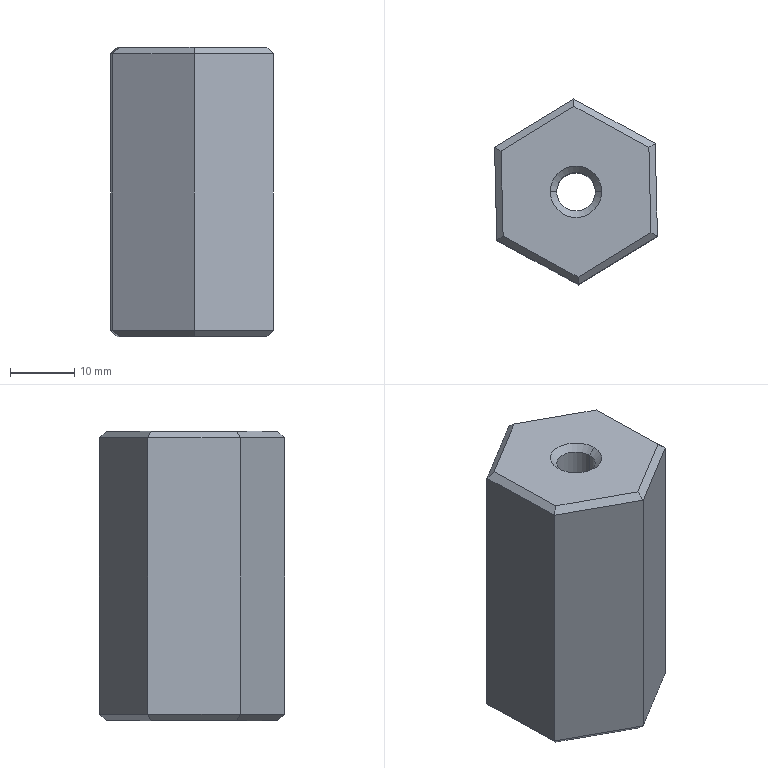Part | STEP file | Sheath | 1 solid | 26 faces | box 25.34 x 28.859 x 45 mm | volume 22979 mm3 | plane 20 | cone 4 | cylinder 2 | commonest cylinder face diameters 6 x2
STEP:
#1=CARTESIAN_POINT('',(3.,0.,1.));
#2=VERTEX_POINT('',#1);
#3=CARTESIAN_POINT('',(-3.,0.,1.));
#4=VERTEX_POINT('',#3);
#5=CARTESIAN_POINT('',(0.,0.,1.));
#6=DIRECTION('',(0.,0.,-1.));
#7=DIRECTION('',(-1.,0.,0.));
#8=AXIS2_PLACEMENT_3D('',#5,#6,#7);
#9=CIRCLE('',#8,3.);
#10=EDGE_CURVE('',#2,#4,#9,.T.);
#11=ORIENTED_EDGE('',*,*,#10,.F.);
#12=CARTESIAN_POINT('',(4.,0.,0.));
#13=VERTEX_POINT('',#12);
#14=CARTESIAN_POINT('',(4.,0.,0.));
#15=DIRECTION('',(0.7071,0.,-0.7071));
#16=VECTOR('',#15,1000.);
#17=LINE('',#14,#16);
#18=EDGE_CURVE('',#2,#13,#17,.T.);
#19=ORIENTED_EDGE('',*,*,#18,.T.);
#20=CARTESIAN_POINT('',(-4.,0.,0.));
#21=VERTEX_POINT('',#20);
#22=CARTESIAN_POINT('',(0.,0.,0.));
#23=DIRECTION('',(0.,0.,-1.));
#24=DIRECTION('',(-1.,0.,0.));
#25=AXIS2_PLACEMENT_3D('',#22,#23,#24);
#26=CIRCLE('',#25,4.);
#27=EDGE_CURVE('',#13,#21,#26,.T.);
#28=ORIENTED_EDGE('',*,*,#27,.T.);
#29=CARTESIAN_POINT('',(-4.,0.,0.));
#30=DIRECTION('',(-0.7071,0.,-0.7071));
#31=VECTOR('',#30,1000.);
#32=LINE('',#29,#31);
#33=EDGE_CURVE('',#4,#21,#32,.T.);
#34=ORIENTED_EDGE('',*,*,#33,.F.);
#35=EDGE_LOOP('',(#11,#19,#28,#34));
#36=FACE_OUTER_BOUND('',#35,.T.);
#37=CARTESIAN_POINT('',(0.,0.,0.));
#38=DIRECTION('',(0.,0.,-1.));
#39=DIRECTION('',(-1.,0.,0.));
#40=AXIS2_PLACEMENT_3D('',#37,#38,#39);
#41=CONICAL_SURFACE('',#40,4.,0.7854);
#42=ADVANCED_FACE('',(#36),#41,.F.);
#43=CARTESIAN_POINT('',(-3.,0.,44.));
#44=VERTEX_POINT('',#43);
#45=CARTESIAN_POINT('',(3.,0.,44.));
#46=VERTEX_POINT('',#45);
#47=CARTESIAN_POINT('',(0.,0.,44.));
#48=DIRECTION('',(0.,0.,1.));
#49=DIRECTION('',(1.,0.,0.));
#50=AXIS2_PLACEMENT_3D('',#47,#48,#49);
#51=CIRCLE('',#50,3.);
#52=EDGE_CURVE('',#44,#46,#51,.T.);
#53=ORIENTED_EDGE('',*,*,#52,.F.);
#54=CARTESIAN_POINT('',(-4.,0.,45.));
#55=VERTEX_POINT('',#54);
#56=CARTESIAN_POINT('',(-4.,0.,45.));
#57=DIRECTION('',(-0.7071,0.,0.7071));
#58=VECTOR('',#57,1000.);
#59=LINE('',#56,#58);
#60=EDGE_CURVE('',#44,#55,#59,.T.);
#61=ORIENTED_EDGE('',*,*,#60,.T.);
#62=CARTESIAN_POINT('',(4.,0.,45.));
#63=VERTEX_POINT('',#62);
#64=CARTESIAN_POINT('',(0.,0.,45.));
#65=DIRECTION('',(0.,0.,-1.));
#66=DIRECTION('',(1.,0.,0.));
#67=AXIS2_PLACEMENT_3D('',#64,#65,#66);
#68=CIRCLE('',#67,4.);
#69=EDGE_CURVE('',#63,#55,#68,.T.);
#70=ORIENTED_EDGE('',*,*,#69,.F.);
#71=CARTESIAN_POINT('',(4.,0.,45.));
#72=DIRECTION('',(0.7071,0.,0.7071));
#73=VECTOR('',#72,1000.);
#74=LINE('',#71,#73);
#75=EDGE_CURVE('',#46,#63,#74,.T.);
#76=ORIENTED_EDGE('',*,*,#75,.F.);
#77=EDGE_LOOP('',(#53,#61,#70,#76));
#78=FACE_OUTER_BOUND('',#77,.T.);
#79=CARTESIAN_POINT('',(0.,0.,45.));
#80=DIRECTION('',(0.,0.,1.));
#81=DIRECTION('',(1.,0.,0.));
#82=AXIS2_PLACEMENT_3D('',#79,#80,#81);
#83=CONICAL_SURFACE('',#82,4.,0.7854);
#84=ADVANCED_FACE('',(#78),#83,.F.);
#85=ORIENTED_EDGE('',*,*,#52,.T.);
#86=CARTESIAN_POINT('',(3.,0.,45.));
#87=DIRECTION('',(0.,0.,-1.));
#88=VECTOR('',#87,1000.);
#89=LINE('',#86,#88);
#90=EDGE_CURVE('',#46,#2,#89,.T.);
#91=ORIENTED_EDGE('',*,*,#90,.T.);
#92=ORIENTED_EDGE('',*,*,#10,.T.);
#93=CARTESIAN_POINT('',(-3.,0.,45.));
#94=DIRECTION('',(0.,0.,-1.));
#95=VECTOR('',#94,1000.);
#96=LINE('',#93,#95);
#97=EDGE_CURVE('',#44,#4,#96,.T.);
#98=ORIENTED_EDGE('',*,*,#97,.F.);
#99=EDGE_LOOP('',(#85,#91,#92,#98));
#100=FACE_OUTER_BOUND('',#99,.T.);
#101=CARTESIAN_POINT('',(0.,0.,45.));
#102=DIRECTION('',(0.,0.,-1.));
#103=DIRECTION('',(-1.,0.,0.));
#104=AXIS2_PLACEMENT_3D('',#101,#102,#103);
#105=CYLINDRICAL_SURFACE('',#104,3.);
#106=ADVANCED_FACE('',(#100),#105,.F.);
#107=CARTESIAN_POINT('',(12.323,7.516,1.));
#108=VERTEX_POINT('',#107);
#109=CARTESIAN_POINT('',(12.67,-6.914,1.));
#110=VERTEX_POINT('',#109);
#111=CARTESIAN_POINT('',(12.67,-6.914,1.));
#112=DIRECTION('',(0.02408,-0.9997,0.));
#113=VECTOR('',#112,1000.);
#114=LINE('',#111,#113);
#115=EDGE_CURVE('',#108,#110,#114,.T.);
#116=ORIENTED_EDGE('',*,*,#115,.F.);
#117=CARTESIAN_POINT('',(12.323,7.516,44.));
#118=VERTEX_POINT('',#117);
#119=CARTESIAN_POINT('',(12.323,7.516,45.));
#120=DIRECTION('',(0.,0.,-1.));
#121=VECTOR('',#120,1000.);
#122=LINE('',#119,#121);
#123=EDGE_CURVE('',#118,#108,#122,.T.);
#124=ORIENTED_EDGE('',*,*,#123,.F.);
#125=CARTESIAN_POINT('',(12.67,-6.914,44.));
#126=VERTEX_POINT('',#125);
#127=CARTESIAN_POINT('',(12.67,-6.914,44.));
#128=DIRECTION('',(-0.02408,0.9997,0.));
#129=VECTOR('',#128,1000.);
#130=LINE('',#127,#129);
#131=EDGE_CURVE('',#126,#118,#130,.T.);
#132=ORIENTED_EDGE('',*,*,#131,.F.);
#133=CARTESIAN_POINT('',(12.67,-6.914,45.));
#134=DIRECTION('',(0.,0.,1.));
#135=VECTOR('',#134,1000.);
#136=LINE('',#133,#135);
#137=EDGE_CURVE('',#110,#126,#136,.T.);
#138=ORIENTED_EDGE('',*,*,#137,.F.);
#139=EDGE_LOOP('',(#116,#124,#132,#138));
#140=FACE_OUTER_BOUND('',#139,.T.);
#141=CARTESIAN_POINT('',(12.67,-6.914,45.));
#142=DIRECTION('',(-0.9997,-0.02408,0.));
#143=DIRECTION('',(0.02408,-0.9997,0.));
#144=AXIS2_PLACEMENT_3D('',#141,#142,#143);
#145=PLANE('',#144);
#146=ADVANCED_FACE('',(#140),#145,.F.);
#147=CARTESIAN_POINT('',(0.3475,-14.43,1.));
#148=VERTEX_POINT('',#147);
#149=CARTESIAN_POINT('',(0.3475,-14.43,1.));
#150=DIRECTION('',(-0.8537,-0.5207,0.));
#151=VECTOR('',#150,1000.);
#152=LINE('',#149,#151);
#153=EDGE_CURVE('',#110,#148,#152,.T.);
#154=ORIENTED_EDGE('',*,*,#153,.F.);
#155=ORIENTED_EDGE('',*,*,#137,.T.);
#156=CARTESIAN_POINT('',(0.3475,-14.43,44.));
#157=VERTEX_POINT('',#156);
#158=CARTESIAN_POINT('',(0.3475,-14.43,44.));
#159=DIRECTION('',(0.8537,0.5207,0.));
#160=VECTOR('',#159,1000.);
#161=LINE('',#158,#160);
#162=EDGE_CURVE('',#157,#126,#161,.T.);
#163=ORIENTED_EDGE('',*,*,#162,.F.);
#164=CARTESIAN_POINT('',(0.3475,-14.43,45.));
#165=DIRECTION('',(0.,0.,1.));
#166=VECTOR('',#165,1000.);
#167=LINE('',#164,#166);
#168=EDGE_CURVE('',#148,#157,#167,.T.);
#169=ORIENTED_EDGE('',*,*,#168,.F.);
#170=EDGE_LOOP('',(#154,#155,#163,#169));
#171=FACE_OUTER_BOUND('',#170,.T.);
#172=CARTESIAN_POINT('',(0.3475,-14.43,45.));
#173=DIRECTION('',(-0.5207,0.8537,0.));
#174=DIRECTION('',(-0.8537,-0.5207,0.));
#175=AXIS2_PLACEMENT_3D('',#172,#173,#174);
#176=PLANE('',#175);
#177=ADVANCED_FACE('',(#171),#176,.F.);
#178=CARTESIAN_POINT('',(11.337,6.914,0.));
#179=VERTEX_POINT('',#178);
#180=CARTESIAN_POINT('',(11.657,-6.361,0.));
#181=VERTEX_POINT('',#180);
#182=CARTESIAN_POINT('',(11.337,6.914,0.));
#183=DIRECTION('',(0.02408,-0.9997,0.));
#184=VECTOR('',#183,1000.);
#185=LINE('',#182,#184);
#186=EDGE_CURVE('',#179,#181,#185,.T.);
#187=ORIENTED_EDGE('',*,*,#186,.F.);
#188=CARTESIAN_POINT('',(11.337,6.914,0.));
#189=DIRECTION('',(0.6454,0.3936,0.6547));
#190=VECTOR('',#189,1000.);
#191=LINE('',#188,#190);
#192=EDGE_CURVE('',#179,#108,#191,.T.);
#193=ORIENTED_EDGE('',*,*,#192,.T.);
#194=ORIENTED_EDGE('',*,*,#115,.T.);
#195=CARTESIAN_POINT('',(11.657,-6.361,0.));
#196=DIRECTION('',(0.6636,-0.3621,0.6547));
#197=VECTOR('',#196,1000.);
#198=LINE('',#195,#197);
#199=EDGE_CURVE('',#181,#110,#198,.T.);
#200=ORIENTED_EDGE('',*,*,#199,.F.);
#201=EDGE_LOOP('',(#187,#193,#194,#200));
#202=FACE_OUTER_BOUND('',#201,.T.);
#203=CARTESIAN_POINT('',(12.67,-6.914,1.));
#204=DIRECTION('',(-0.7069,-0.01702,0.7071));
#205=DIRECTION('',(0.7072,0.,0.707));
#206=AXIS2_PLACEMENT_3D('',#203,#204,#205);
#207=PLANE('',#206);
#208=ADVANCED_FACE('',(#202),#207,.F.);
#209=CARTESIAN_POINT('',(-0.3475,14.43,1.));
#210=VERTEX_POINT('',#209);
#211=CARTESIAN_POINT('',(12.323,7.516,1.));
#212=DIRECTION('',(0.8778,-0.479,0.));
#213=VECTOR('',#212,1000.);
#214=LINE('',#211,#213);
#215=EDGE_CURVE('',#210,#108,#214,.T.);
#216=ORIENTED_EDGE('',*,*,#215,.F.);
#217=CARTESIAN_POINT('',(-0.3475,14.43,44.));
#218=VERTEX_POINT('',#217);
#219=CARTESIAN_POINT('',(-0.3475,14.43,45.));
#220=DIRECTION('',(0.,0.,-1.));
#221=VECTOR('',#220,1000.);
#222=LINE('',#219,#221);
#223=EDGE_CURVE('',#218,#210,#222,.T.);
#224=ORIENTED_EDGE('',*,*,#223,.F.);
#225=CARTESIAN_POINT('',(12.323,7.516,44.));
#226=DIRECTION('',(-0.8778,0.479,0.));
#227=VECTOR('',#226,1000.);
#228=LINE('',#225,#227);
#229=EDGE_CURVE('',#118,#218,#228,.T.);
#230=ORIENTED_EDGE('',*,*,#229,.F.);
#231=ORIENTED_EDGE('',*,*,#123,.T.);
#232=EDGE_LOOP('',(#216,#224,#230,#231));
#233=FACE_OUTER_BOUND('',#232,.T.);
#234=CARTESIAN_POINT('',(12.323,7.516,45.));
#235=DIRECTION('',(-0.479,-0.8778,0.));
#236=DIRECTION('',(0.8778,-0.479,0.));
#237=AXIS2_PLACEMENT_3D('',#234,#235,#236);
#238=PLANE('',#237);
#239=ADVANCED_FACE('',(#233),#238,.F.);
#240=CARTESIAN_POINT('',(11.657,-6.361,45.));
#241=VERTEX_POINT('',#240);
#242=CARTESIAN_POINT('',(11.657,-6.361,45.));
#243=DIRECTION('',(0.6636,-0.3621,-0.6547));
#244=VECTOR('',#243,1000.);
#245=LINE('',#242,#244);
#246=EDGE_CURVE('',#241,#126,#245,.T.);
#247=ORIENTED_EDGE('',*,*,#246,.T.);
#248=ORIENTED_EDGE('',*,*,#131,.T.);
#249=CARTESIAN_POINT('',(11.337,6.914,45.));
#250=VERTEX_POINT('',#249);
#251=CARTESIAN_POINT('',(12.323,7.516,44.));
#252=DIRECTION('',(-0.6454,-0.3936,0.6547));
#253=VECTOR('',#252,1000.);
#254=LINE('',#251,#253);
#255=EDGE_CURVE('',#118,#250,#254,.T.);
#256=ORIENTED_EDGE('',*,*,#255,.T.);
#257=CARTESIAN_POINT('',(11.337,6.914,45.));
#258=DIRECTION('',(0.02408,-0.9997,0.));
#259=VECTOR('',#258,1000.);
#260=LINE('',#257,#259);
#261=EDGE_CURVE('',#250,#241,#260,.T.);
#262=ORIENTED_EDGE('',*,*,#261,.T.);
#263=EDGE_LOOP('',(#247,#248,#256,#262));
#264=FACE_OUTER_BOUND('',#263,.T.);
#265=CARTESIAN_POINT('',(11.67,-6.938,45.));
#266=DIRECTION('',(0.7069,0.01702,0.7071));
#267=DIRECTION('',(0.7072,0.,-0.707));
#268=AXIS2_PLACEMENT_3D('',#265,#266,#267);
#269=PLANE('',#268);
#270=ADVANCED_FACE('',(#264),#269,.T.);
#271=CARTESIAN_POINT('',(-12.323,-7.516,1.));
#272=VERTEX_POINT('',#271);
#273=CARTESIAN_POINT('',(-12.323,-7.516,1.));
#274=DIRECTION('',(-0.8778,0.479,0.));
#275=VECTOR('',#274,1000.);
#276=LINE('',#273,#275);
#277=EDGE_CURVE('',#148,#272,#276,.T.);
#278=ORIENTED_EDGE('',*,*,#277,.F.);
#279=ORIENTED_EDGE('',*,*,#168,.T.);
#280=CARTESIAN_POINT('',(-12.323,-7.516,44.));
#281=VERTEX_POINT('',#280);
#282=CARTESIAN_POINT('',(-12.323,-7.516,44.));
#283=DIRECTION('',(0.8778,-0.479,0.));
#284=VECTOR('',#283,1000.);
#285=LINE('',#282,#284);
#286=EDGE_CURVE('',#281,#157,#285,.T.);
#287=ORIENTED_EDGE('',*,*,#286,.F.);
#288=CARTESIAN_POINT('',(-12.323,-7.516,45.));
#289=DIRECTION('',(0.,0.,1.));
#290=VECTOR('',#289,1000.);
#291=LINE('',#288,#290);
#292=EDGE_CURVE('',#272,#281,#291,.T.);
#293=ORIENTED_EDGE('',*,*,#292,.F.);
#294=EDGE_LOOP('',(#278,#279,#287,#293));
#295=FACE_OUTER_BOUND('',#294,.T.);
#296=CARTESIAN_POINT('',(-12.323,-7.516,45.));
#297=DIRECTION('',(0.479,0.8778,0.));
#298=DIRECTION('',(-0.8778,0.479,0.));
#299=AXIS2_PLACEMENT_3D('',#296,#297,#298);
#300=PLANE('',#299);
#301=ADVANCED_FACE('',(#295),#300,.F.);
#302=CARTESIAN_POINT('',(0.3197,-13.275,0.));
#303=VERTEX_POINT('',#302);
#304=CARTESIAN_POINT('',(11.657,-6.361,0.));
#305=DIRECTION('',(-0.8537,-0.5207,0.));
#306=VECTOR('',#305,1000.);
#307=LINE('',#304,#306);
#308=EDGE_CURVE('',#181,#303,#307,.T.);
#309=ORIENTED_EDGE('',*,*,#308,.F.);
#310=ORIENTED_EDGE('',*,*,#199,.T.);
#311=ORIENTED_EDGE('',*,*,#153,.T.);
#312=CARTESIAN_POINT('',(0.3197,-13.275,0.));
#313=DIRECTION('',(0.0182,-0.7557,0.6547));
#314=VECTOR('',#313,1000.);
#315=LINE('',#312,#314);
#316=EDGE_CURVE('',#303,#148,#315,.T.);
#317=ORIENTED_EDGE('',*,*,#316,.F.);
#318=EDGE_LOOP('',(#309,#310,#311,#317));
#319=FACE_OUTER_BOUND('',#318,.T.);
#320=CARTESIAN_POINT('',(0.3475,-14.43,1.));
#321=DIRECTION('',(-0.3682,0.6037,0.7071));
#322=DIRECTION('',(0.,-0.7605,0.6493));
#323=AXIS2_PLACEMENT_3D('',#320,#321,#322);
#324=PLANE('',#323);
#325=ADVANCED_FACE('',(#319),#324,.F.);
#326=CARTESIAN_POINT('',(0.3197,-13.275,45.));
#327=VERTEX_POINT('',#326);
#328=CARTESIAN_POINT('',(0.3197,-13.275,45.));
#329=DIRECTION('',(0.0182,-0.7557,-0.6547));
#330=VECTOR('',#329,1000.);
#331=LINE('',#328,#330);
#332=EDGE_CURVE('',#327,#157,#331,.T.);
#333=ORIENTED_EDGE('',*,*,#332,.T.);
#334=ORIENTED_EDGE('',*,*,#162,.T.);
#335=ORIENTED_EDGE('',*,*,#246,.F.);
#336=CARTESIAN_POINT('',(11.657,-6.361,45.));
#337=DIRECTION('',(-0.8537,-0.5207,0.));
#338=VECTOR('',#337,1000.);
#339=LINE('',#336,#338);
#340=EDGE_CURVE('',#241,#327,#339,.T.);
#341=ORIENTED_EDGE('',*,*,#340,.T.);
#342=EDGE_LOOP('',(#333,#334,#335,#341));
#343=FACE_OUTER_BOUND('',#342,.T.);
#344=CARTESIAN_POINT('',(12.149,-6.06,45.));
#345=DIRECTION('',(0.3682,-0.6037,0.7071));
#346=DIRECTION('',(0.,-0.7605,-0.6493));
#347=AXIS2_PLACEMENT_3D('',#344,#345,#346);
#348=PLANE('',#347);
#349=ADVANCED_FACE('',(#343),#348,.T.);
#350=ORIENTED_EDGE('',*,*,#186,.T.);
#351=ORIENTED_EDGE('',*,*,#308,.T.);
#352=CARTESIAN_POINT('',(-11.337,-6.914,0.));
#353=VERTEX_POINT('',#352);
#354=CARTESIAN_POINT('',(-11.337,-6.914,0.));
#355=DIRECTION('',(0.8778,-0.479,0.));
#356=VECTOR('',#355,1000.);
#357=LINE('',#354,#356);
#358=EDGE_CURVE('',#353,#303,#357,.T.);
#359=ORIENTED_EDGE('',*,*,#358,.F.);
#360=CARTESIAN_POINT('',(-11.657,6.361,0.));
#361=VERTEX_POINT('',#360);
#362=CARTESIAN_POINT('',(-11.657,6.361,0.));
#363=DIRECTION('',(0.02408,-0.9997,0.));
#364=VECTOR('',#363,1000.);
#365=LINE('',#362,#364);
#366=EDGE_CURVE('',#361,#353,#365,.T.);
#367=ORIENTED_EDGE('',*,*,#366,.F.);
#368=CARTESIAN_POINT('',(-0.3197,13.275,0.));
#369=VERTEX_POINT('',#368);
#370=CARTESIAN_POINT('',(-0.3197,13.275,0.));
#371=DIRECTION('',(-0.8537,-0.5207,0.));
#372=VECTOR('',#371,1000.);
#373=LINE('',#370,#372);
#374=EDGE_CURVE('',#369,#361,#373,.T.);
#375=ORIENTED_EDGE('',*,*,#374,.F.);
#376=CARTESIAN_POINT('',(11.337,6.914,0.));
#377=DIRECTION('',(-0.8778,0.479,0.));
#378=VECTOR('',#377,1000.);
#379=LINE('',#376,#378);
#380=EDGE_CURVE('',#179,#369,#379,.T.);
#381=ORIENTED_EDGE('',*,*,#380,.F.);
#382=EDGE_LOOP('',(#350,#351,#359,#367,#375,#381));
#383=FACE_OUTER_BOUND('',#382,.T.);
#384=CARTESIAN_POINT('',(0.,0.,0.));
#385=DIRECTION('',(0.,0.,-1.));
#386=DIRECTION('',(-1.,0.,0.));
#387=AXIS2_PLACEMENT_3D('',#384,#385,#386);
#388=CIRCLE('',#387,4.);
#389=EDGE_CURVE('',#21,#13,#388,.T.);
#390=ORIENTED_EDGE('',*,*,#389,.F.);
#391=ORIENTED_EDGE('',*,*,#27,.F.);
#392=EDGE_LOOP('',(#390,#391));
#393=FACE_BOUND('',#392,.T.);
#394=CARTESIAN_POINT('',(12.67,-6.914,0.));
#395=DIRECTION('',(0.,0.,1.));
#396=DIRECTION('',(1.,0.,0.));
#397=AXIS2_PLACEMENT_3D('',#394,#395,#396);
#398=PLANE('',#397);
#399=ADVANCED_FACE('',(#383,#393),#398,.F.);
#400=ORIENTED_EDGE('',*,*,#215,.T.);
#401=ORIENTED_EDGE('',*,*,#192,.F.);
#402=ORIENTED_EDGE('',*,*,#380,.T.);
#403=CARTESIAN_POINT('',(-0.3475,14.43,1.));
#404=DIRECTION('',(0.0182,-0.7557,-0.6547));
#405=VECTOR('',#404,1000.);
#406=LINE('',#403,#405);
#407=EDGE_CURVE('',#210,#369,#406,.T.);
#408=ORIENTED_EDGE('',*,*,#407,.F.);
#409=EDGE_LOOP('',(#400,#401,#402,#408));
#410=FACE_OUTER_BOUND('',#409,.T.);
#411=CARTESIAN_POINT('',(12.323,7.516,1.));
#412=DIRECTION('',(-0.3387,-0.6207,0.7071));
#413=DIRECTION('',(0.,-0.7515,-0.6597));
#414=AXIS2_PLACEMENT_3D('',#411,#412,#413);
#415=PLANE('',#414);
#416=ADVANCED_FACE('',(#410),#415,.F.);
#417=CARTESIAN_POINT('',(-12.67,6.914,1.));
#418=VERTEX_POINT('',#417);
#419=CARTESIAN_POINT('',(-0.3475,14.43,1.));
#420=DIRECTION('',(0.8537,0.5207,0.));
#421=VECTOR('',#420,1000.);
#422=LINE('',#419,#421);
#423=EDGE_CURVE('',#418,#210,#422,.T.);
#424=ORIENTED_EDGE('',*,*,#423,.F.);
#425=CARTESIAN_POINT('',(-12.67,6.914,44.));
#426=VERTEX_POINT('',#425);
#427=CARTESIAN_POINT('',(-12.67,6.914,45.));
#428=DIRECTION('',(0.,0.,-1.));
#429=VECTOR('',#428,1000.);
#430=LINE('',#427,#429);
#431=EDGE_CURVE('',#426,#418,#430,.T.);
#432=ORIENTED_EDGE('',*,*,#431,.F.);
#433=CARTESIAN_POINT('',(-0.3475,14.43,44.));
#434=DIRECTION('',(-0.8537,-0.5207,0.));
#435=VECTOR('',#434,1000.);
#436=LINE('',#433,#435);
#437=EDGE_CURVE('',#218,#426,#436,.T.);
#438=ORIENTED_EDGE('',*,*,#437,.F.);
#439=ORIENTED_EDGE('',*,*,#223,.T.);
#440=EDGE_LOOP('',(#424,#432,#438,#439));
#441=FACE_OUTER_BOUND('',#440,.T.);
#442=CARTESIAN_POINT('',(-0.3475,14.43,45.));
#443=DIRECTION('',(0.5207,-0.8537,0.));
#444=DIRECTION('',(0.8537,0.5207,0.));
#445=AXIS2_PLACEMENT_3D('',#442,#443,#444);
#446=PLANE('',#445);
#447=ADVANCED_FACE('',(#441),#446,.F.);
#448=CARTESIAN_POINT('',(-0.3197,13.275,45.));
#449=VERTEX_POINT('',#448);
#450=CARTESIAN_POINT('',(-0.3475,14.43,44.));
#451=DIRECTION('',(0.0182,-0.7557,0.6547));
#452=VECTOR('',#451,1000.);
#453=LINE('',#450,#452);
#454=EDGE_CURVE('',#218,#449,#453,.T.);
#455=ORIENTED_EDGE('',*,*,#454,.T.);
#456=CARTESIAN_POINT('',(-0.3197,13.275,45.));
#457=DIRECTION('',(0.8778,-0.479,0.));
#458=VECTOR('',#457,1000.);
#459=LINE('',#456,#458);
#460=EDGE_CURVE('',#449,#250,#459,.T.);
#461=ORIENTED_EDGE('',*,*,#460,.T.);
#462=ORIENTED_EDGE('',*,*,#255,.F.);
#463=ORIENTED_EDGE('',*,*,#229,.T.);
#464=EDGE_LOOP('',(#455,#461,#462,#463));
#465=FACE_OUTER_BOUND('',#464,.T.);
#466=CARTESIAN_POINT('',(18.179,3.181,45.));
#467=DIRECTION('',(0.3387,0.6207,0.7071));
#468=DIRECTION('',(0.,-0.7515,0.6597));
#469=AXIS2_PLACEMENT_3D('',#466,#467,#468);
#470=PLANE('',#469);
#471=ADVANCED_FACE('',(#465),#470,.T.);
#472=ORIENTED_EDGE('',*,*,#460,.F.);
#473=CARTESIAN_POINT('',(-11.657,6.361,45.));
#474=VERTEX_POINT('',#473);
#475=CARTESIAN_POINT('',(-0.3197,13.275,45.));
#476=DIRECTION('',(-0.8537,-0.5207,0.));
#477=VECTOR('',#476,1000.);
#478=LINE('',#475,#477);
#479=EDGE_CURVE('',#449,#474,#478,.T.);
#480=ORIENTED_EDGE('',*,*,#479,.T.);
#481=CARTESIAN_POINT('',(-11.337,-6.914,45.));
#482=VERTEX_POINT('',#481);
#483=CARTESIAN_POINT('',(-11.657,6.361,45.));
#484=DIRECTION('',(0.02408,-0.9997,0.));
#485=VECTOR('',#484,1000.);
#486=LINE('',#483,#485);
#487=EDGE_CURVE('',#474,#482,#486,.T.);
#488=ORIENTED_EDGE('',*,*,#487,.T.);
#489=CARTESIAN_POINT('',(-11.337,-6.914,45.));
#490=DIRECTION('',(0.8778,-0.479,0.));
#491=VECTOR('',#490,1000.);
#492=LINE('',#489,#491);
#493=EDGE_CURVE('',#482,#327,#492,.T.);
#494=ORIENTED_EDGE('',*,*,#493,.T.);
#495=ORIENTED_EDGE('',*,*,#340,.F.);
#496=ORIENTED_EDGE('',*,*,#261,.F.);
#497=EDGE_LOOP('',(#472,#480,#488,#494,#495,#496));
#498=FACE_OUTER_BOUND('',#497,.T.);
#499=ORIENTED_EDGE('',*,*,#69,.T.);
#500=CARTESIAN_POINT('',(0.,0.,45.));
#501=DIRECTION('',(0.,0.,-1.));
#502=DIRECTION('',(1.,0.,0.));
#503=AXIS2_PLACEMENT_3D('',#500,#501,#502);
#504=CIRCLE('',#503,4.);
#505=EDGE_CURVE('',#55,#63,#504,.T.);
#506=ORIENTED_EDGE('',*,*,#505,.T.);
#507=EDGE_LOOP('',(#499,#506));
#508=FACE_BOUND('',#507,.T.);
#509=CARTESIAN_POINT('',(12.67,-6.914,45.));
#510=DIRECTION('',(0.,0.,1.));
#511=DIRECTION('',(1.,0.,0.));
#512=AXIS2_PLACEMENT_3D('',#509,#510,#511);
#513=PLANE('',#512);
#514=ADVANCED_FACE('',(#498,#508),#513,.T.);
#515=CARTESIAN_POINT('',(-12.67,6.914,1.));
#516=DIRECTION('',(-0.02408,0.9997,0.));
#517=VECTOR('',#516,1000.);
#518=LINE('',#515,#517);
#519=EDGE_CURVE('',#272,#418,#518,.T.);
#520=ORIENTED_EDGE('',*,*,#519,.F.);
#521=ORIENTED_EDGE('',*,*,#292,.T.);
#522=CARTESIAN_POINT('',(-12.67,6.914,44.));
#523=DIRECTION('',(0.02408,-0.9997,0.));
#524=VECTOR('',#523,1000.);
#525=LINE('',#522,#524);
#526=EDGE_CURVE('',#426,#281,#525,.T.);
#527=ORIENTED_EDGE('',*,*,#526,.F.);
#528=ORIENTED_EDGE('',*,*,#431,.T.);
#529=EDGE_LOOP('',(#520,#521,#527,#528));
#530=FACE_OUTER_BOUND('',#529,.T.);
#531=CARTESIAN_POINT('',(-12.67,6.914,45.));
#532=DIRECTION('',(0.9997,0.02408,0.));
#533=DIRECTION('',(-0.02408,0.9997,0.));
#534=AXIS2_PLACEMENT_3D('',#531,#532,#533);
#535=PLANE('',#534);
#536=ADVANCED_FACE('',(#530),#535,.F.);
#537=ORIENTED_EDGE('',*,*,#358,.T.);
#538=ORIENTED_EDGE('',*,*,#316,.T.);
#539=ORIENTED_EDGE('',*,*,#277,.T.);
#540=CARTESIAN_POINT('',(-11.337,-6.914,0.));
#541=DIRECTION('',(-0.6454,-0.3936,0.6547));
#542=VECTOR('',#541,1000.);
#543=LINE('',#540,#542);
#544=EDGE_CURVE('',#353,#272,#543,.T.);
#545=ORIENTED_EDGE('',*,*,#544,.F.);
#546=EDGE_LOOP('',(#537,#538,#539,#545));
#547=FACE_OUTER_BOUND('',#546,.T.);
#548=CARTESIAN_POINT('',(-12.323,-7.516,1.));
#549=DIRECTION('',(0.3387,0.6207,0.7071));
#550=DIRECTION('',(0.,-0.7515,0.6597));
#551=AXIS2_PLACEMENT_3D('',#548,#549,#550);
#552=PLANE('',#551);
#553=ADVANCED_FACE('',(#547),#552,.F.);
#554=ORIENTED_EDGE('',*,*,#332,.F.);
#555=ORIENTED_EDGE('',*,*,#493,.F.);
#556=CARTESIAN_POINT('',(-11.337,-6.914,45.));
#557=DIRECTION('',(-0.6454,-0.3936,-0.6547));
#558=VECTOR('',#557,1000.);
#559=LINE('',#556,#558);
#560=EDGE_CURVE('',#482,#281,#559,.T.);
#561=ORIENTED_EDGE('',*,*,#560,.T.);
#562=ORIENTED_EDGE('',*,*,#286,.T.);
#563=EDGE_LOOP('',(#554,#555,#561,#562));
#564=FACE_OUTER_BOUND('',#563,.T.);
#565=CARTESIAN_POINT('',(7.162,-17.009,45.));
#566=DIRECTION('',(-0.3387,-0.6207,0.7071));
#567=DIRECTION('',(0.,-0.7515,-0.6597));
#568=AXIS2_PLACEMENT_3D('',#565,#566,#567);
#569=PLANE('',#568);
#570=ADVANCED_FACE('',(#564),#569,.T.);
#571=ORIENTED_EDGE('',*,*,#366,.T.);
#572=ORIENTED_EDGE('',*,*,#544,.T.);
#573=ORIENTED_EDGE('',*,*,#519,.T.);
#574=CARTESIAN_POINT('',(-11.657,6.361,0.));
#575=DIRECTION('',(-0.6636,0.3621,0.6547));
#576=VECTOR('',#575,1000.);
#577=LINE('',#574,#576);
#578=EDGE_CURVE('',#361,#418,#577,.T.);
#579=ORIENTED_EDGE('',*,*,#578,.F.);
#580=EDGE_LOOP('',(#571,#572,#573,#579));
#581=FACE_OUTER_BOUND('',#580,.T.);
#582=CARTESIAN_POINT('',(-12.67,6.914,1.));
#583=DIRECTION('',(0.7069,0.01702,0.7071));
#584=DIRECTION('',(0.7072,0.,-0.707));
#585=AXIS2_PLACEMENT_3D('',#582,#583,#584);
#586=PLANE('',#585);
#587=ADVANCED_FACE('',(#581),#586,.F.);
#588=ORIENTED_EDGE('',*,*,#423,.T.);
#589=ORIENTED_EDGE('',*,*,#407,.T.);
#590=ORIENTED_EDGE('',*,*,#374,.T.);
#591=ORIENTED_EDGE('',*,*,#578,.T.);
#592=EDGE_LOOP('',(#588,#589,#590,#591));
#593=FACE_OUTER_BOUND('',#592,.T.);
#594=CARTESIAN_POINT('',(-0.3475,14.43,1.));
#595=DIRECTION('',(0.3682,-0.6037,0.7071));
#596=DIRECTION('',(0.,-0.7605,-0.6493));
#597=AXIS2_PLACEMENT_3D('',#594,#595,#596);
#598=PLANE('',#597);
#599=ADVANCED_FACE('',(#593),#598,.F.);
#600=ORIENTED_EDGE('',*,*,#18,.F.);
#601=CARTESIAN_POINT('',(0.,0.,1.));
#602=DIRECTION('',(0.,0.,-1.));
#603=DIRECTION('',(-1.,0.,0.));
#604=AXIS2_PLACEMENT_3D('',#601,#602,#603);
#605=CIRCLE('',#604,3.);
#606=EDGE_CURVE('',#4,#2,#605,.T.);
#607=ORIENTED_EDGE('',*,*,#606,.F.);
#608=ORIENTED_EDGE('',*,*,#33,.T.);
#609=ORIENTED_EDGE('',*,*,#389,.T.);
#610=EDGE_LOOP('',(#600,#607,#608,#609));
#611=FACE_OUTER_BOUND('',#610,.T.);
#612=CARTESIAN_POINT('',(0.,0.,0.));
#613=DIRECTION('',(0.,0.,-1.));
#614=DIRECTION('',(-1.,0.,0.));
#615=AXIS2_PLACEMENT_3D('',#612,#613,#614);
#616=CONICAL_SURFACE('',#615,4.,0.7854);
#617=ADVANCED_FACE('',(#611),#616,.F.);
#618=CARTESIAN_POINT('',(-12.67,6.914,44.));
#619=DIRECTION('',(0.6636,-0.3621,0.6547));
#620=VECTOR('',#619,1000.);
#621=LINE('',#618,#620);
#622=EDGE_CURVE('',#426,#474,#621,.T.);
#623=ORIENTED_EDGE('',*,*,#622,.T.);
#624=ORIENTED_EDGE('',*,*,#479,.F.);
#625=ORIENTED_EDGE('',*,*,#454,.F.);
#626=ORIENTED_EDGE('',*,*,#437,.T.);
#627=EDGE_LOOP('',(#623,#624,#625,#626));
#628=FACE_OUTER_BOUND('',#627,.T.);
#629=CARTESIAN_POINT('',(0.1732,13.576,45.));
#630=DIRECTION('',(-0.3682,0.6037,0.7071));
#631=DIRECTION('',(0.,-0.7605,0.6493));
#632=AXIS2_PLACEMENT_3D('',#629,#630,#631);
#633=PLANE('',#632);
#634=ADVANCED_FACE('',(#628),#633,.T.);
#635=ORIENTED_EDGE('',*,*,#560,.F.);
#636=ORIENTED_EDGE('',*,*,#487,.F.);
#637=ORIENTED_EDGE('',*,*,#622,.F.);
#638=ORIENTED_EDGE('',*,*,#526,.T.);
#639=EDGE_LOOP('',(#635,#636,#637,#638));
#640=FACE_OUTER_BOUND('',#639,.T.);
#641=CARTESIAN_POINT('',(-11.323,-7.492,45.));
#642=DIRECTION('',(-0.7069,-0.01702,0.7071));
#643=DIRECTION('',(0.7072,0.,0.707));
#644=AXIS2_PLACEMENT_3D('',#641,#642,#643);
#645=PLANE('',#644);
#646=ADVANCED_FACE('',(#640),#645,.T.);
#647=ORIENTED_EDGE('',*,*,#60,.F.);
#648=CARTESIAN_POINT('',(0.,0.,44.));
#649=DIRECTION('',(0.,0.,1.));
#650=DIRECTION('',(1.,0.,0.));
#651=AXIS2_PLACEMENT_3D('',#648,#649,#650);
#652=CIRCLE('',#651,3.);
#653=EDGE_CURVE('',#46,#44,#652,.T.);
#654=ORIENTED_EDGE('',*,*,#653,.F.);
#655=ORIENTED_EDGE('',*,*,#75,.T.);
#656=ORIENTED_EDGE('',*,*,#505,.F.);
#657=EDGE_LOOP('',(#647,#654,#655,#656));
#658=FACE_OUTER_BOUND('',#657,.T.);
#659=CARTESIAN_POINT('',(0.,0.,45.));
#660=DIRECTION('',(0.,0.,1.));
#661=DIRECTION('',(1.,0.,0.));
#662=AXIS2_PLACEMENT_3D('',#659,#660,#661);
#663=CONICAL_SURFACE('',#662,4.,0.7854);
#664=ADVANCED_FACE('',(#658),#663,.F.);
#665=ORIENTED_EDGE('',*,*,#90,.F.);
#666=ORIENTED_EDGE('',*,*,#653,.T.);
#667=ORIENTED_EDGE('',*,*,#97,.T.);
#668=ORIENTED_EDGE('',*,*,#606,.T.);
#669=EDGE_LOOP('',(#665,#666,#667,#668));
#670=FACE_OUTER_BOUND('',#669,.T.);
#671=CARTESIAN_POINT('',(0.,0.,45.));
#672=DIRECTION('',(0.,0.,-1.));
#673=DIRECTION('',(-1.,0.,0.));
#674=AXIS2_PLACEMENT_3D('',#671,#672,#673);
#675=CYLINDRICAL_SURFACE('',#674,3.);
#676=ADVANCED_FACE('',(#670),#675,.F.);
#677=CLOSED_SHELL('',(#42,#84,#106,#146,#177,#208,#239,#270,#301,#325,#349,#399,#416,#447,#471,#514,#536,#553,#570,#587,#599,#617,#634,#646,#664,#676));
#678=MANIFOLD_SOLID_BREP('',#677);
#679=CARTESIAN_POINT('',(0.,0.,0.));
#680=DIRECTION('',(0.,0.,1.));
#681=DIRECTION('',(1.,0.,0.));
#682=AXIS2_PLACEMENT_3D('',#679,#680,#681);
#683=(LENGTH_UNIT()NAMED_UNIT(*)SI_UNIT(.MILLI.,.METRE.));
#684=UNCERTAINTY_MEASURE_WITH_UNIT(LENGTH_MEASURE(0.00001),#683,'','');
#685=(NAMED_UNIT(*)PLANE_ANGLE_UNIT()SI_UNIT($,.RADIAN.));
#686=(NAMED_UNIT(*)SI_UNIT($,.STERADIAN.)SOLID_ANGLE_UNIT());
#687=(GEOMETRIC_REPRESENTATION_CONTEXT(3)GLOBAL_UNCERTAINTY_ASSIGNED_CONTEXT((#684))GLOBAL_UNIT_ASSIGNED_CONTEXT((#683,#685,#686))REPRESENTATION_CONTEXT('',''));
#688=ADVANCED_BREP_SHAPE_REPRESENTATION('',(#678,#682),#687);